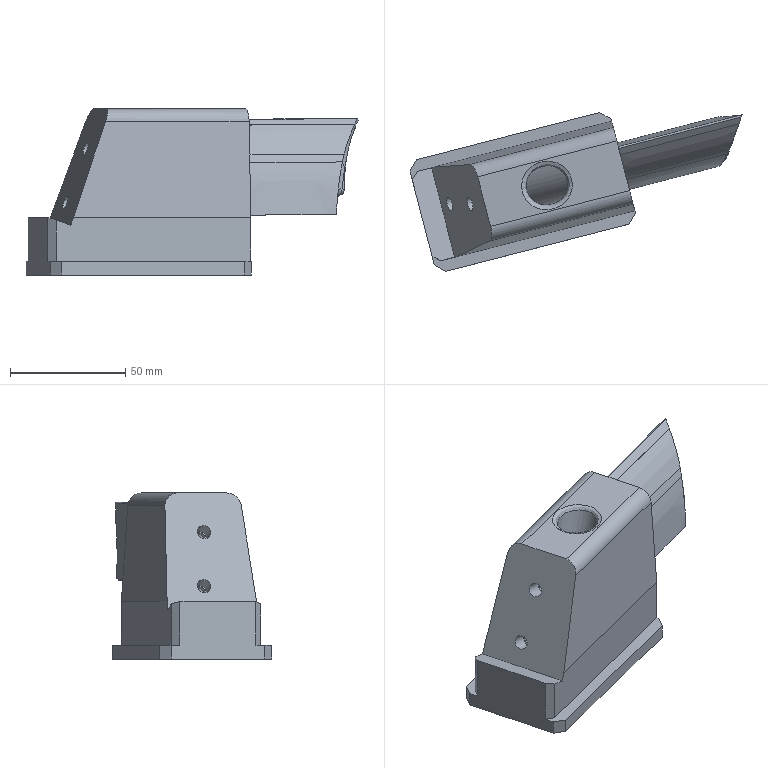Part | STEP file | 车灯-后视镜_id78_x_t | 1 solid | 93 faces | box 143.857 x 68.896 x 72 mm | volume 222992 mm3 | spline 43 | plane 27 | other 11 | cylinder 8 | cone 2 | sphere 2 | commonest cylinder face diameters 5.1 x2 6 x2 12 x2 1 x1 17 x1